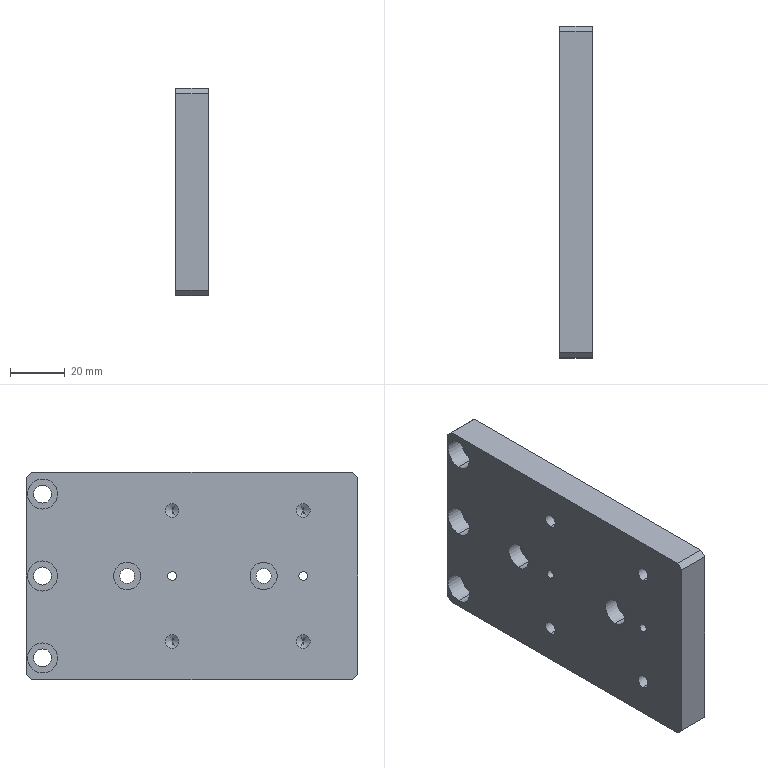Part | SolidWorks | features HoleWzd 4, Chamfer 1, Extrusion 1 | 1 solid | 55 faces | box 12 x 121.5 x 76 mm | volume 106329 mm3 | cylinder 32 | plane 15 | cone 8 | commonest cylinder face diameters 5 x8 6.6 x6 11 x6 3.3 x4 5.5 x4 10 x4